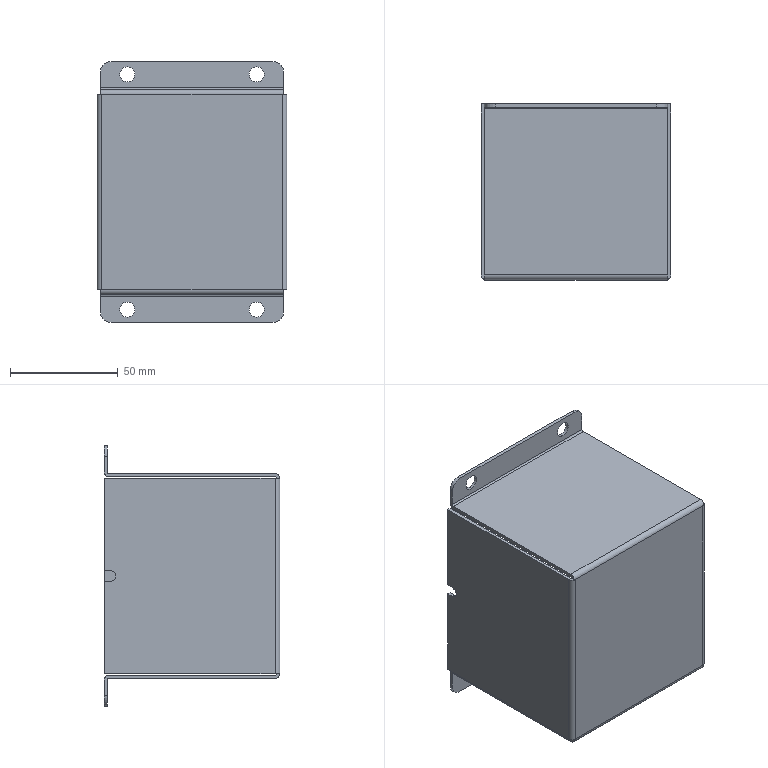Part | SolidWorks | features BaseBody 1 | 1 solid | 61 faces | box 88 x 81.5 x 121 mm | volume 56566 mm3 | plane 33 | cylinder 28 | commonest cylinder face diameters 7 x8 1.473 x6 4.473 x6 10 x4 5 x2 22.5 x2